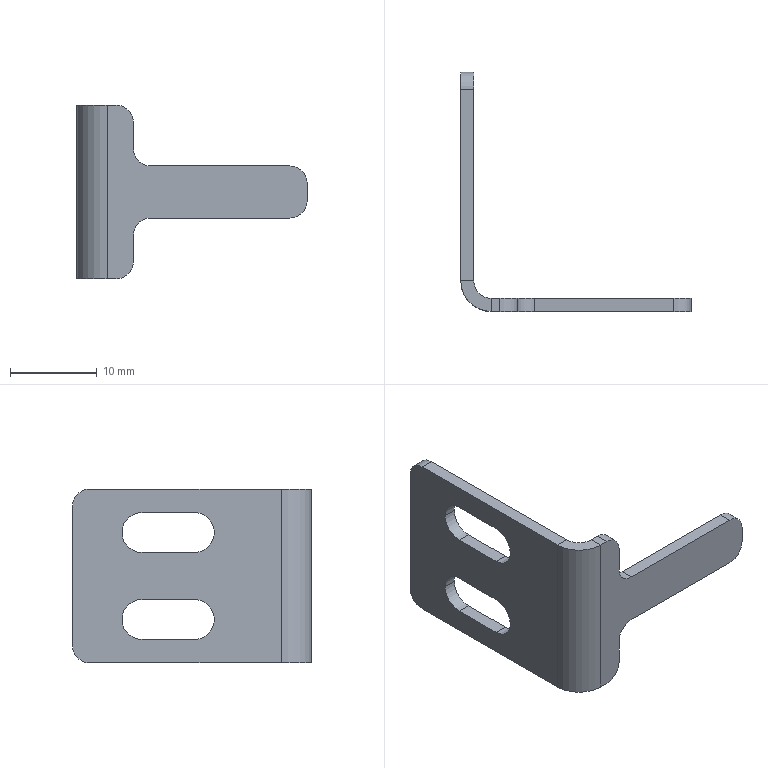Part | STEP file | M-05-748A_default | 1 solid | 36 faces | box 26.5 x 27.5 x 20 mm | volume 981.783 mm3 | plane 20 | cylinder 16 | commonest cylinder face diameters 4 x9 4.6 x6 7 x1